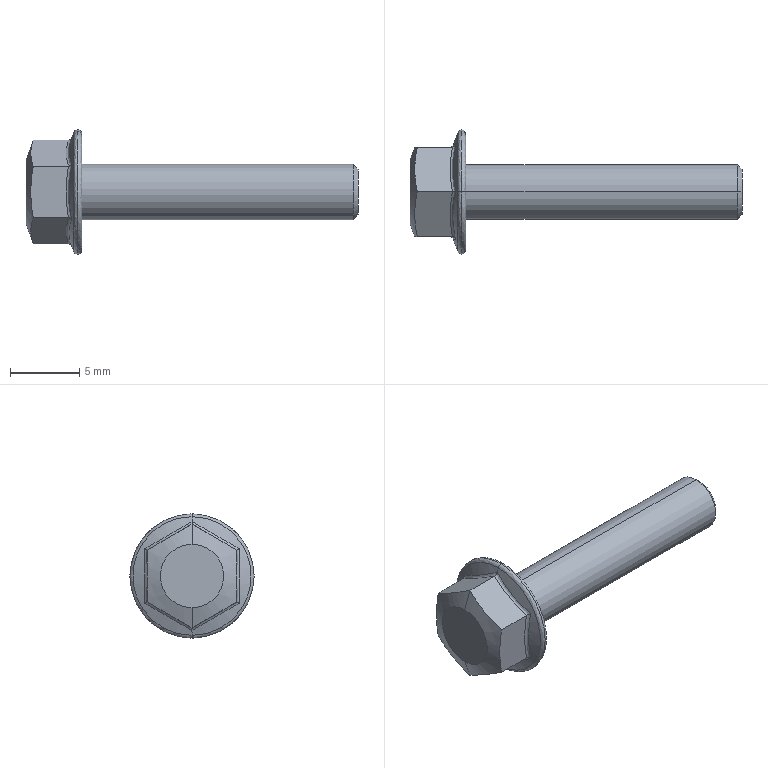Part | SolidWorks | features BaseBody 1, Scale 1 | 1 solid | 27 faces | box 24.05 x 9 x 9 mm | volume 413.187 mm3 | spline 10 | plane 9 | cone 6 | cylinder 2 | commonest cylinder face diameters 4 x2